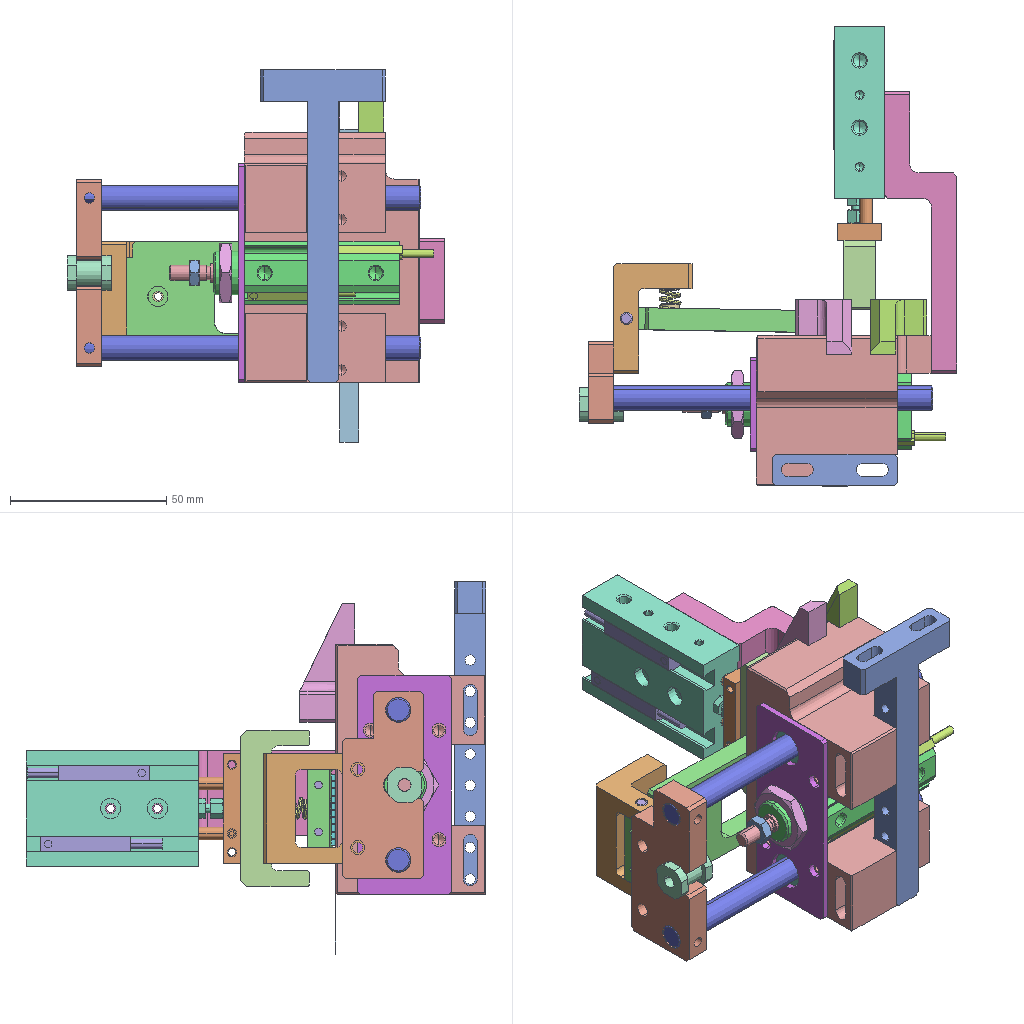Assembly | SolidWorks | 30 different items | 44 placed | box 121 x 147 x 119 mm
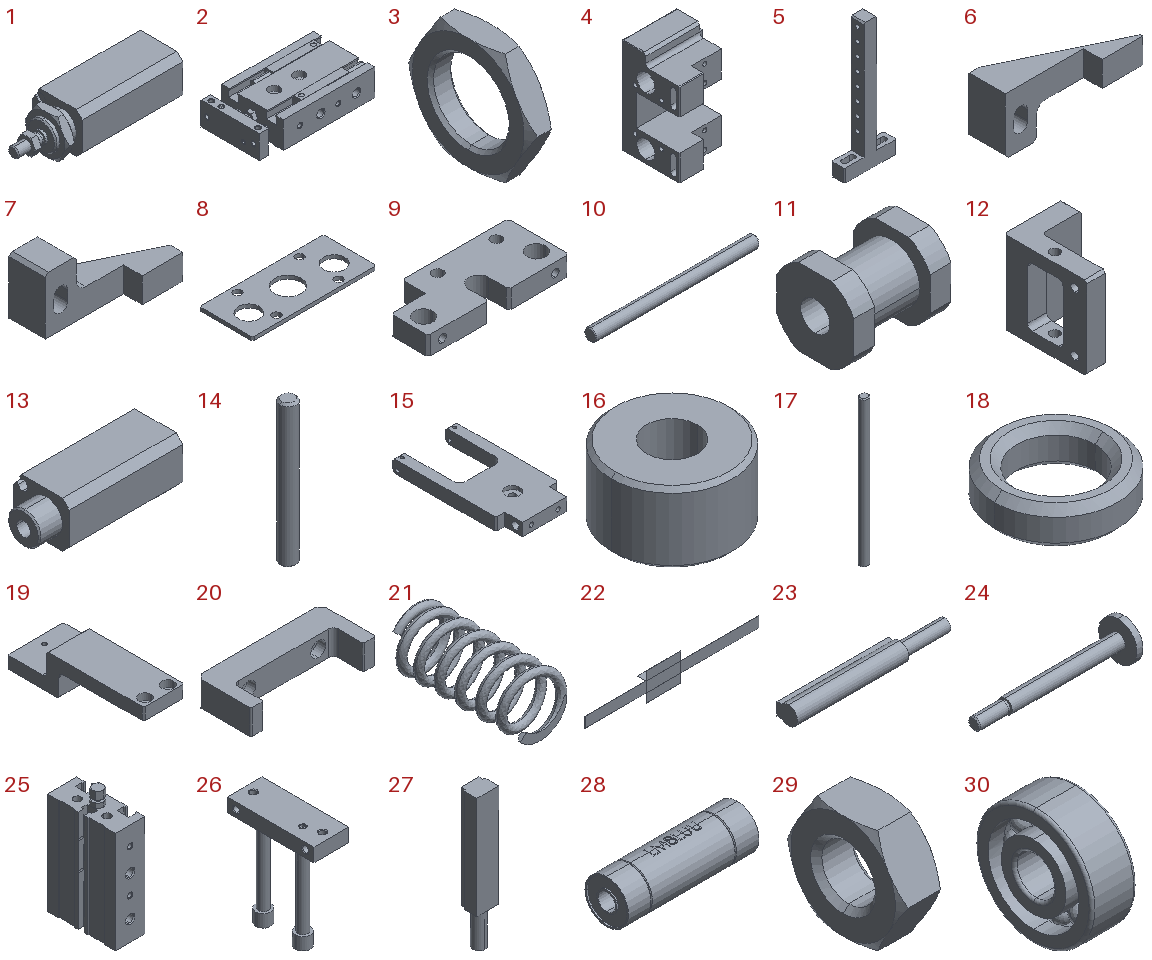Parts list (item | name | quantity | parent item | size | volume | features):
1 | (subassembly) | x1 | - | 84.5 x 25.47 x 20 mm | 20169 mm3 | features AEMSimFeature 1
2 | (subassembly) | x1 | - | 68.5 x 37 x 16.2 mm | 31090 mm3 | features AEMSimFeature 1
3 | - | x1 | in 1 | 4 x 21.939 x 19 mm | 699.231 mm3 | features RefAxis 3, RevCut 2, 3DProfileFeature 1, Extrusion 1
4 | - | x1 | - | 56 x 48 x 80 mm | 94389 mm3 | features HoleWzd 9, ICE 9, Chamfer 3, Fillet 2, CutThin 1, Extrusion 1, LPattern 1
5 | - | x1 | - | 40 x 10 x 100 mm | 11505 mm3 | features ICE 3, Chamfer 1, Extrusion 1, HoleWzd 1
6 | - | x1 | - | 38 x 17.5 x 18 mm | 3099 mm3 | features ICE 4, Chamfer 2, Extrusion 1, Fillet 1
7 | - | x1 | - | 38 x 17.5 x 18 mm | 3099 mm3 | features ICE 4, Chamfer 2, Extrusion 1, Fillet 1
8 | - | x1 | - | 70 x 30 x 2 mm | 3263 mm3 | features Chamfer 1, Extrusion 1, HoleWzd 1
9 | - | x1 | - | 60 x 26 x 8 mm | 9318 mm3 | features ICE 3, HoleWzd 2, Chamfer 1, Extrusion 1
10 | - | x2 | - | 110 x 8 x 8 mm | 5509 mm3 | features Chamfer 1, ICE 1, Revolution 1
11 | - | x1 | - | 14 x 11 x 11 mm | 848.048 mm3 | features HoleWzd 1, ICE 1, Revolution 1
12 | - | x1 | - | 25 x 35 x 35 mm | 11031 mm3 | features ICE 3, HoleWzd 2, Chamfer 1, Extrusion 1, Fillet 1
13 | - | x1 | in 1 | 59.5 x 24.5 x 20 mm | 16440 mm3 | features RefAxis 18, 3DProfileFeature 6, RevCut 3, Extrusion 1, Revolution 1
14 | - | x1 | - | 4 x 4 x 35 mm | 416.091 mm3 | features Chamfer 1, Extrusion 1, ICE 1
15 | - | x1 | - | 35 x 68 x 7 mm | 9996 mm3 | features ICE 4, HoleWzd 3, Fillet 2, Chamfer 1, Extrusion 1
16 | - | x2 | - | 6 x 6 x 3.5 mm | 81.042 mm3 | features Chamfer 1, Extrusion 1, HoleWzd 1
17 | - | x1 | - | 2 x 2 x 35 mm | 109.721 mm3 | features Chamfer 1, Extrusion 1, RefAxis 1
18 | - | x1 | - | 3.3 x 3.3 x 1 mm | 4.411 mm3 | features Chamfer 1, Extrusion 1
19 | - | x1 | - | 37 x 90 x 23 mm | 24810 mm3 | features ICE 3, Chamfer 2, HoleWzd 2, Extrusion 1, Fillet 1
20 | - | x1 | - | 50 x 22 x 10 mm | 5859 mm3 | features Fillet 2, Chamfer 1, Extrusion 1, HoleWzd 1
21 | - | x1 | - | 6.997 x 15.003 x 6.998 mm | 95.492 mm3 | features Helix 1, ICE 1, Sweep 1
22 | - | x1 | - | 100 x 5.02 x 16 mm | 70.4 mm3 | features ICE 2, ExtruThin 1
23 | - | x2 | in 1 | 34.5 x 4.5 x 4 mm | 409.198 mm3 | features RefAxis 3, ICE 2, 3DProfileFeature 1, Extrusion 1
24 | - | x1 | in 1 | 62.5 x 16 x 16 mm | 2081 mm3 | features RefAxis 9, 3DProfileFeature 3, Revolution 3
25 | - | x1 | in 2 | 16 x 37 x 63 mm | 25617 mm3 | features HoleWzd 12, RefAxis 9, 3DProfileFeature 3, RevCut 2, Revolution 2, Extrusion 1, ICE 1
26 | - | x1 | in 2 | 14 x 35 x 41.5 mm | 3580 mm3 | features ICE 4, RevCut 4, RefAxis 3, Revolution 2, 3DProfileFeature 1, Extrusion 1
27 | - | x2 | in 2 | 6.2 x 5 x 39 mm | 946.118 mm3 | features RefAxis 6, 3DProfileFeature 2, Extrusion 1, RevCut 1, Revolution 1
28 | - | x2 | - | 45 x 15 x 15 mm | 6555 mm3 | features Emboss 1, Revolution 1
29 | - | x1 | in 1 | 3.2 x 9.238 x 8 mm | 130.688 mm3 | features RefAxis 3, RevCut 2, 3DProfileFeature 1, Extrusion 1
30 | - | x10 | - | 2.3 x 6 x 6 mm | 42.074 mm3 | features Stock 1
Mates (type | each side: item.copy, entity, surface, feature):
In the top assembly
Parallel | 4.1 face plane Boss-Extrude1 | 6.1 face plane Boss-Extrude1
Coincident | 4.1 face plane Boss-Extrude1 | 6.1 face plane Cut-Extrude2 | 2 times
Coincident | 4.1 face plane Boss-Extrude1 | 7.1 face plane Cut-Extrude2
Coincident | 6.1 face plane Boss-Extrude1 | 7.1 face plane Boss-Extrude1
Concentric | 4.1 face cylinder Cut-Extrude1 | 28.1 face cylinder Revolve1
Concentric | 4.1 face cylinder Cut-Extrude1 | 28.2 face cylinder Revolve1
Concentric | 15.1 face cylinder Cut-Extrude1 | 17.1 face cylinder Boss-Extrude1
Coincident | 15.1 face plane Boss-Extrude1 | 17.1 face plane Boss-Extrude1
Concentric | 14.1 face cylinder Boss-Extrude1 | 15.1 face cylinder Cut-Extrude3
Concentric | 12.1 face cylinder Cut-Extrude2 | 14.1 face cylinder Boss-Extrude1
Coincident | 12.1 face plane Boss-Extrude1 | 14.1 face plane Boss-Extrude1
Coincident | 12.1 face plane Cut-Extrude1 | 15.1 face plane Cut-Extrude2
Coincident | 4.1 face plane Boss-Extrude1 | 22.1 face plane Boss-Extrude1
Parallel | 14.1 face plane Cut-Extrude1 | 15.1 face plane Boss-Extrude1
Coincident | 4.1 face plane Boss-Extrude1 | 8.1 face plane Boss-Extrude1
Concentric | 4.1 face cylinder M4 Tapped Hole6 | 8.1 face cylinder Ø4.5 (4.5) Diameter Hole1 | 2 times
Concentric | 9.1 face cylinder Boss-Extrude1 | 10.1 face cylinder Revolve1
Concentric | 9.1 face cylinder Boss-Extrude1 | 10.2 face cylinder Revolve1
Coincident | 9.1 face plane Boss-Extrude1 | 10.1 face plane Revolve1
Coincident | 9.1 face plane Boss-Extrude1 | 10.2 face plane Revolve1
Coincident | 12.1 face plane Boss-Extrude1 | 9.1 face plane Boss-Extrude1
Concentric | 12.1 face cylinder M4 Tapped Hole1 | 9.1 face cylinder Cut-Extrude3 | 2 times
Concentric | 10.2 face cylinder Revolve1 | 28.2 face cylinder Revolve1
Concentric | 28.1 face cylinder Revolve1 | 10.1 face cylinder Revolve1
Coincident | 11.1 face plane Revolve1 | 9.1 face plane Boss-Extrude1
Coincident | 4.1 face plane Boss-Extrude1 | 19.1 face plane Boss-Extrude1
Concentric | 4.1 face cylinder M4 Tapped Hole5 | 19.1 face cylinder CBORE for M4 Hex Head Bolt1 | 2 times
Coincident | 4.1 face plane Boss-Extrude1 | 28.1 face plane Revolve1
Coincident | 4.1 face plane Boss-Extrude1 | 28.2 face plane Revolve1
Coincident | 4.1 plane | 22.1 plane
Concentric | 12.1 face cylinder Cut-Extrude3 | 16.1 face cylinder Boss-Extrude1
DistanceDim | 7.1 face plane Boss-Extrude1 | 6.1 face plane Boss-Extrude1
Width | 4.1 face plane Cut-Extrude-Thin1 | 4.1 face plane Cut-Extrude-Thin1 | 7.1 face plane Boss-Extrude1 | 6.1 face plane Boss-Extrude1
Concentric | 17.1 face cylinder Boss-Extrude1 | 30.1 face cylinder deep groove ball bearings gb
Coincident | 15.1 face plane Boss-Extrude1 | 30.1 face plane deep groove ball bearings gb
Concentric | 12.1 face cylinder CBORE for M3 Hex Socket Head Cap Screw1 | 16.1 face cylinder Boss-Extrude1
Coincident | 12.1 face plane Cut-Extrude3 | 16.1 face plane Boss-Extrude1
Concentric | 15.1 face cylinder CBORE for M3 Hex Socket Head Cap Screw1 | 16.2 face cylinder Boss-Extrude1
Coincident | 15.1 edge | 16.2 face plane Boss-Extrude1
Concentric | 30.1 face cylinder deep groove ball bearings gb | 18.1 face cylinder Boss-Extrude1
Coincident | 30.2 face plane deep groove ball bearings gb | 18.1 face plane Boss-Extrude1
Tangent | 4.1 face plane Boss-Extrude1 | 30.1 face cylinder deep groove ball bearings gb
Coincident | 8.1 face plane Boss-Extrude1 | 13.1 face plane Boss-Extrude1
Concentric | 8.1 face cylinder Boss-Extrude1 | 13.1 face cylinder Revolve1
Parallel | 4.1 face plane Boss-Extrude2 | 13.1 face plane Boss-Extrude1
LimitDistanceDim | 29.1 face plane Boss-Extrude1 | 11.1 face plane Revolve1
Coincident | 4.1 face plane Boss-Extrude2 | 5.1 face plane Boss-Extrude1
Coincident | 19.1 face plane Boss-Extrude2 | 25.1 face plane Boss-Extrude1
Coincident | 20.1 face plane Boss-Extrude1 | 26.1 face plane Boss-Extrude1
Concentric | 20.1 face cylinder CBORE for M3 Hex Head Bolt1 | 26.1 face cylinder Cut-Revolve2
Concentric | 19.1 face cylinder M3 Tapped Hole1 | 25.1 face cylinder Hole1
Concentric | 19.1 face cylinder M3 Tapped Hole1 | 25.1 face cylinder Hole2
Concentric | 20.1 face cylinder CBORE for M3 Hex Head Bolt1 | 26.1 face cylinder Cut-Revolve1
In subassembly 1
Coincident | 13.2 axis | 24.1 axis | 3 times
PlanarAngleDim | 24.1 plane | 13.2 plane
DistanceDim | 29.2 plane | 24.1 plane
Coincident | 24.1 axis | 29.2 axis | 3 times
PlanarAngleDim | 29.2 plane | 24.1 plane
Coincident | 13.2 axis | 23.1 axis | 3 times
PlanarAngleDim | 23.1 plane | 13.2 plane
Coincident | 13.2 axis | 23.2 axis | 3 times
PlanarAngleDim | 23.2 plane | 13.2 plane
Concentric | 13.2 face cylinder Revolve1 | 3.1 face cylinder Cut-Revolve2
DistanceDim | 13.2 face plane Boss-Extrude1 | 3.1 face plane Boss-Extrude1
In subassembly 2
Coincident | 25.2 axis | 26.2 axis
PlanarAngleDim | 26.2 plane | 25.2 plane
Coincident | 25.2 axis | 27.1 axis
DistanceDim | 27.2 plane | 25.2 plane
Coincident | 25.2 axis | 27.2 axis
PlanarAngleDim | 27.2 plane | 25.2 plane